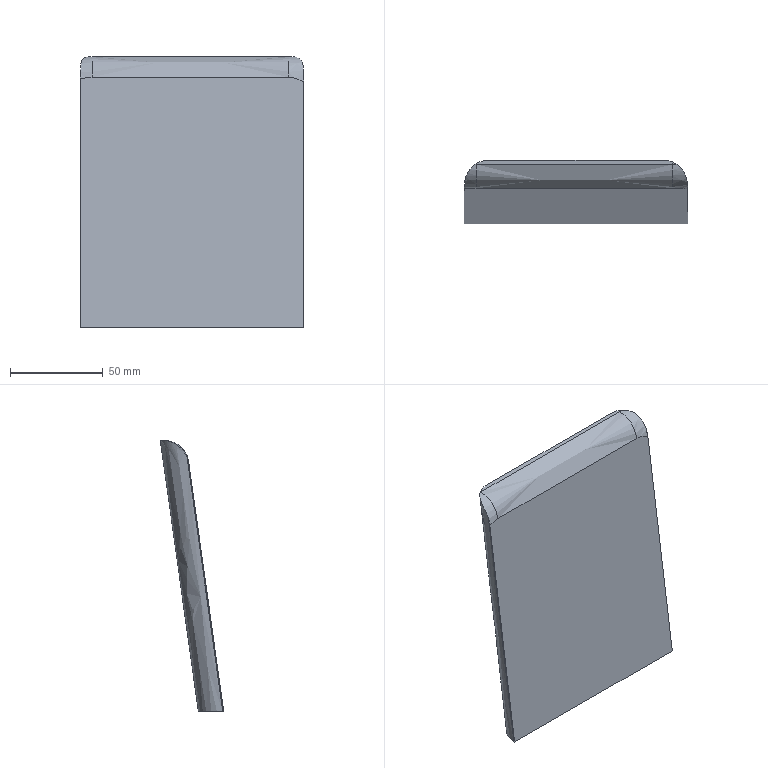Part | STEP file | solid 57 | 1 solid | 13 faces | box 120 x 34.115 x 145.737 mm | volume 224584 mm3 | spline 7 | plane 4 | cylinder 2 | commonest cylinder face diameters 53.689 x1 63.819 x1